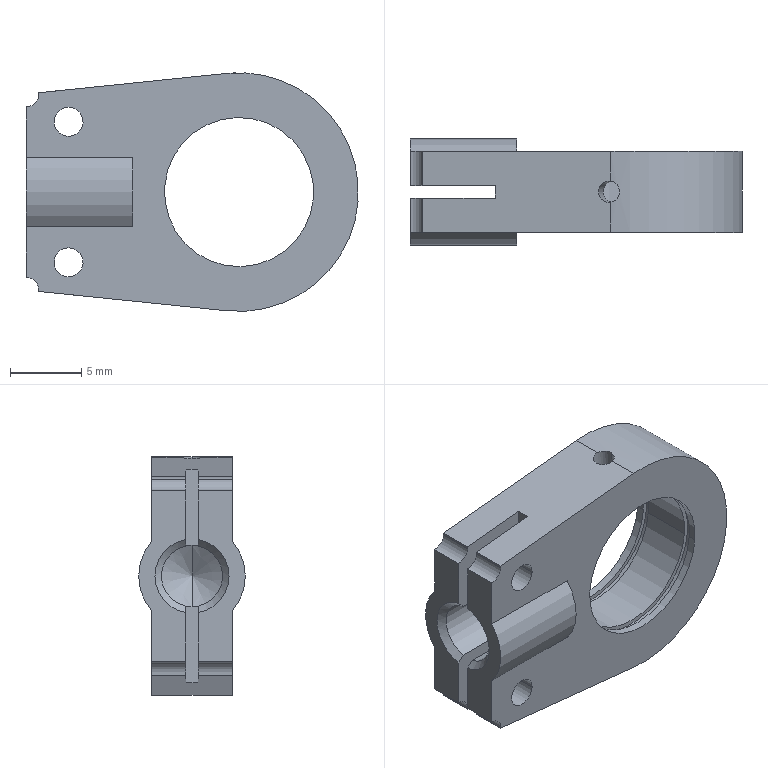Part | STEP file | 2026.6.15-Main Assembly图.sldasm-Part-166 | 1 solid | 56 faces | box 23.4 x 7.5 x 16.8 mm | volume 1292 mm3 | cylinder 34 | plane 18 | cone 4 | commonest cylinder face diameters 1.8 x8 2.04 x8 10.5 x6 11.1 x4 1.5 x2 4.313 x2